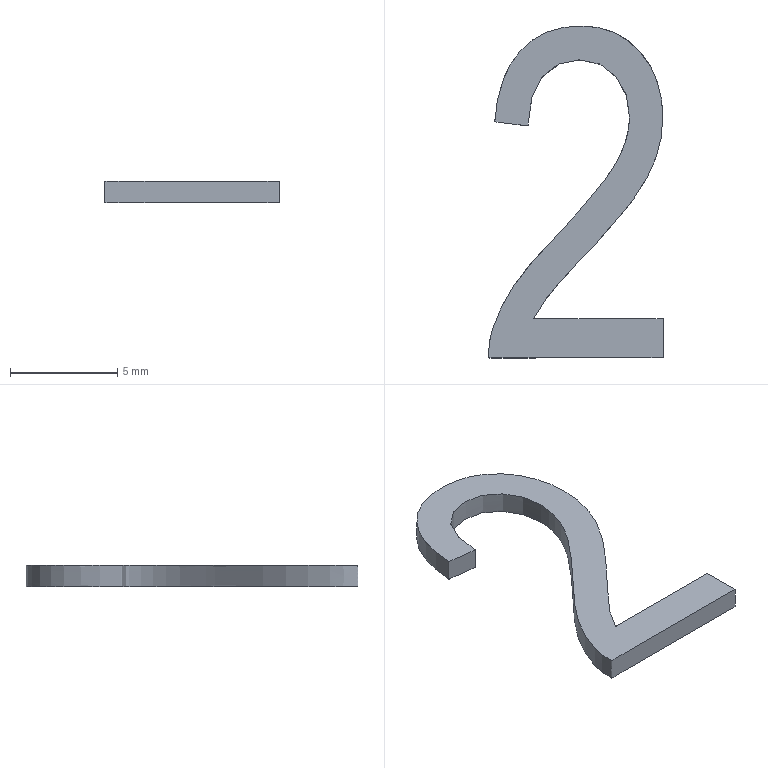Part | STEP file | lll_id1062_x_t | 1 solid | 3 faces | box 8.162 x 15.502 x 1 mm | volume 60.192 mm3 | plane 2 | other 1